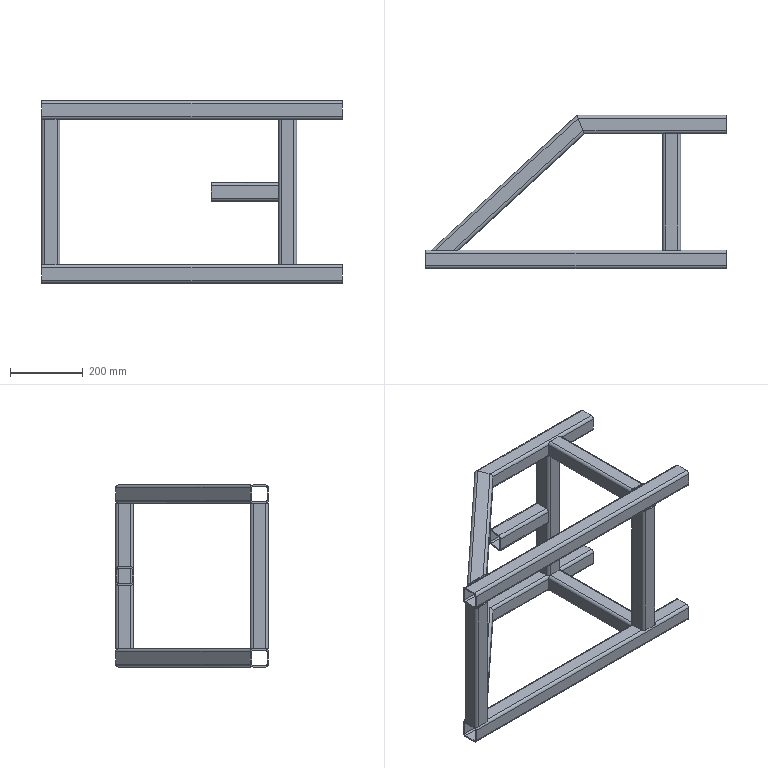Part | SolidWorks | features WeldCornerFeat 3, WeldMemberFeat 2, 3DProfileFeature 1, Cut 1, WeldmentFeature 1 | 12 solids | 216 faces | box 825 x 420 x 500 mm | volume 3812160 mm3 | plane 120 | cylinder 96 | commonest cylinder face diameters 8 x48 16 x48